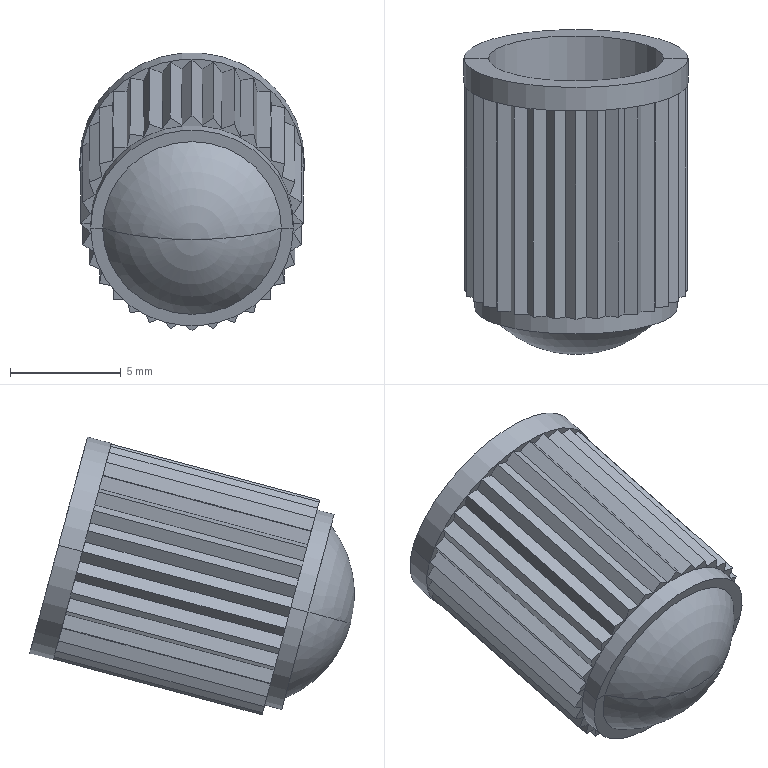Part | STEP file | BREP_3 | 1 solid | 85 faces | box 10.16 x 14.692 x 12.577 mm | volume 395.376 mm3 | plane 75 | cylinder 8 | sphere 2 | commonest cylinder face diameters 6.064 x2 7.94 x2 9.16 x2 10.16 x2